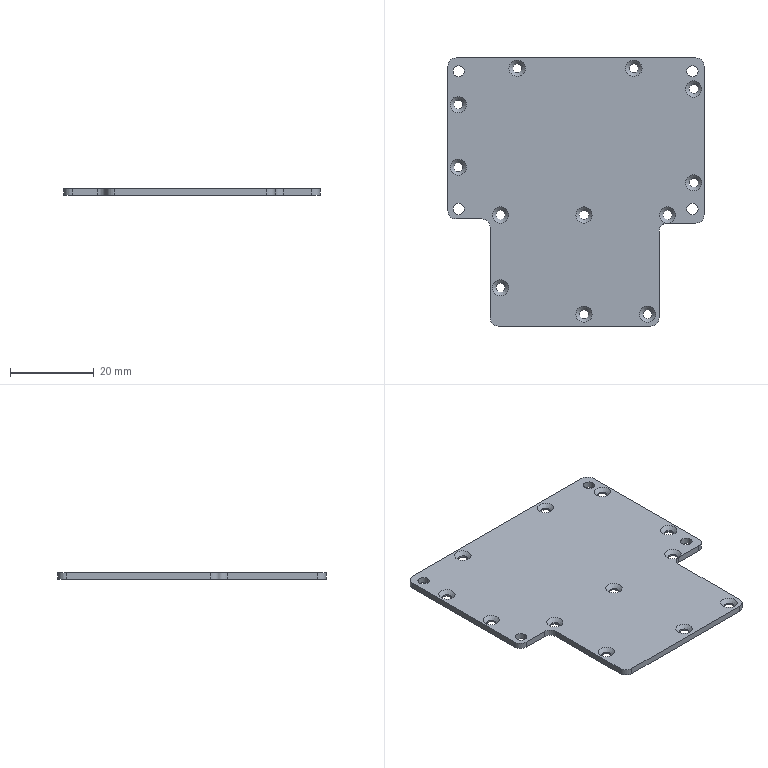Part | STEP file | Front stage cover | 1 solid | 58 faces | box 61.4 x 64.23 x 1.5 mm | volume 4977 mm3 | cylinder 24 | cone 24 | plane 10 | commonest cylinder face diameters 2.2 x12 4 x8 2.7 x4